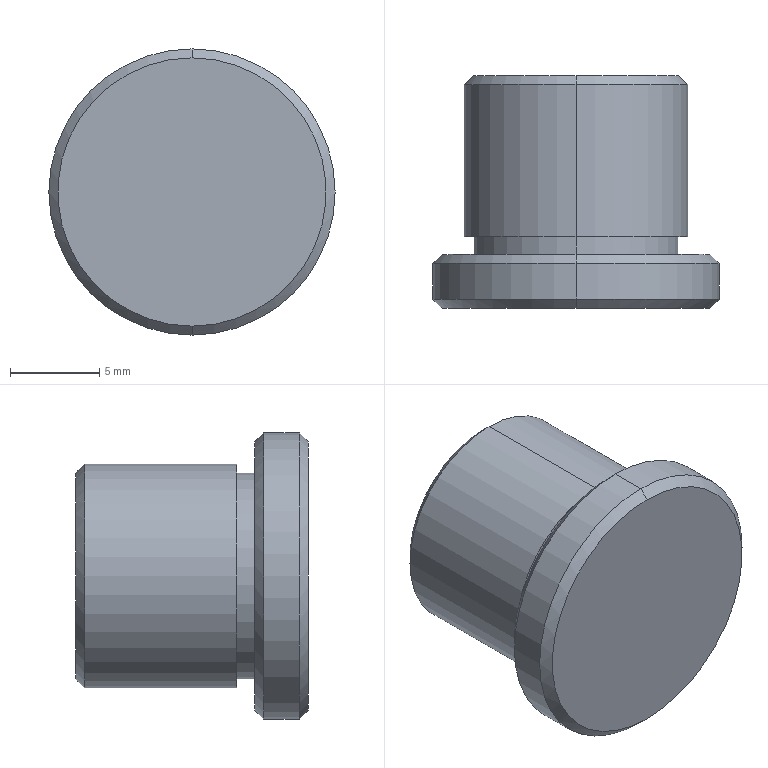Part | SolidWorks | features Chamfer 1, Revolution 1 | 1 solid | 16 faces | box 16 x 13 x 16 mm | volume 1794 mm3 | cone 6 | cylinder 6 | plane 4 | commonest cylinder face diameters 11.5 x2 12.5 x2 16 x2
STEP:
#1=CARTESIAN_POINT('',(74.024,-118.5,5.75));
#2=VERTEX_POINT('',#1);
#3=CARTESIAN_POINT('',(74.024,-118.5,-5.75));
#4=VERTEX_POINT('',#3);
#5=CARTESIAN_POINT('',(74.024,-118.5,0.));
#6=DIRECTION('',(0.,1.,0.));
#7=DIRECTION('',(0.,0.,-1.));
#8=AXIS2_PLACEMENT_3D('',#5,#6,#7);
#9=CIRCLE('',#8,5.75);
#10=EDGE_CURVE('',#2,#4,#9,.T.);
#11=ORIENTED_EDGE('',*,*,#10,.F.);
#12=CARTESIAN_POINT('',(74.024,-119.,6.25));
#13=VERTEX_POINT('',#12);
#14=CARTESIAN_POINT('',(74.024,-118.5,5.75));
#15=DIRECTION('',(0.,-0.7071,0.7071));
#16=VECTOR('',#15,1000.);
#17=LINE('',#14,#16);
#18=EDGE_CURVE('',#2,#13,#17,.T.);
#19=ORIENTED_EDGE('',*,*,#18,.T.);
#20=CARTESIAN_POINT('',(74.024,-119.,-6.25));
#21=VERTEX_POINT('',#20);
#22=CARTESIAN_POINT('',(74.024,-119.,0.));
#23=DIRECTION('',(0.,-1.,0.));
#24=DIRECTION('',(0.,0.,-1.));
#25=AXIS2_PLACEMENT_3D('',#22,#23,#24);
#26=CIRCLE('',#25,6.25);
#27=EDGE_CURVE('',#21,#13,#26,.T.);
#28=ORIENTED_EDGE('',*,*,#27,.F.);
#29=CARTESIAN_POINT('',(74.024,-118.5,-5.75));
#30=DIRECTION('',(0.,-0.7071,-0.7071));
#31=VECTOR('',#30,1000.);
#32=LINE('',#29,#31);
#33=EDGE_CURVE('',#4,#21,#32,.T.);
#34=ORIENTED_EDGE('',*,*,#33,.F.);
#35=EDGE_LOOP('',(#11,#19,#28,#34));
#36=FACE_OUTER_BOUND('',#35,.T.);
#37=CARTESIAN_POINT('',(74.024,-118.5,0.));
#38=DIRECTION('',(0.,-1.,0.));
#39=DIRECTION('',(0.,0.,-1.));
#40=AXIS2_PLACEMENT_3D('',#37,#38,#39);
#41=CONICAL_SURFACE('',#40,5.75,0.7854);
#42=ADVANCED_FACE('',(#36),#41,.T.);
#43=CARTESIAN_POINT('',(74.024,-131.5,-7.5));
#44=VERTEX_POINT('',#43);
#45=CARTESIAN_POINT('',(74.024,-131.5,7.5));
#46=VERTEX_POINT('',#45);
#47=CARTESIAN_POINT('',(74.024,-131.5,0.));
#48=DIRECTION('',(0.,-1.,0.));
#49=DIRECTION('',(0.,0.,1.));
#50=AXIS2_PLACEMENT_3D('',#47,#48,#49);
#51=CIRCLE('',#50,7.5);
#52=EDGE_CURVE('',#44,#46,#51,.T.);
#53=ORIENTED_EDGE('',*,*,#52,.F.);
#54=CARTESIAN_POINT('',(74.024,-131.,-8.));
#55=VERTEX_POINT('',#54);
#56=CARTESIAN_POINT('',(74.024,-131.,-8.));
#57=DIRECTION('',(0.,0.7071,-0.7071));
#58=VECTOR('',#57,1000.);
#59=LINE('',#56,#58);
#60=EDGE_CURVE('',#44,#55,#59,.T.);
#61=ORIENTED_EDGE('',*,*,#60,.T.);
#62=CARTESIAN_POINT('',(74.024,-131.,8.));
#63=VERTEX_POINT('',#62);
#64=CARTESIAN_POINT('',(74.024,-131.,0.));
#65=DIRECTION('',(0.,1.,0.));
#66=DIRECTION('',(0.,0.,1.));
#67=AXIS2_PLACEMENT_3D('',#64,#65,#66);
#68=CIRCLE('',#67,8.);
#69=EDGE_CURVE('',#63,#55,#68,.T.);
#70=ORIENTED_EDGE('',*,*,#69,.F.);
#71=CARTESIAN_POINT('',(74.024,-131.,8.));
#72=DIRECTION('',(0.,0.7071,0.7071));
#73=VECTOR('',#72,1000.);
#74=LINE('',#71,#73);
#75=EDGE_CURVE('',#46,#63,#74,.T.);
#76=ORIENTED_EDGE('',*,*,#75,.F.);
#77=EDGE_LOOP('',(#53,#61,#70,#76));
#78=FACE_OUTER_BOUND('',#77,.T.);
#79=CARTESIAN_POINT('',(74.024,-131.,0.));
#80=DIRECTION('',(0.,1.,0.));
#81=DIRECTION('',(0.,0.,1.));
#82=AXIS2_PLACEMENT_3D('',#79,#80,#81);
#83=CONICAL_SURFACE('',#82,8.,0.7854);
#84=ADVANCED_FACE('',(#78),#83,.T.);
#85=CARTESIAN_POINT('',(74.024,-128.5,7.5));
#86=VERTEX_POINT('',#85);
#87=CARTESIAN_POINT('',(74.024,-128.5,-7.5));
#88=VERTEX_POINT('',#87);
#89=CARTESIAN_POINT('',(74.024,-128.5,0.));
#90=DIRECTION('',(0.,1.,0.));
#91=DIRECTION('',(0.,0.,-1.));
#92=AXIS2_PLACEMENT_3D('',#89,#90,#91);
#93=CIRCLE('',#92,7.5);
#94=EDGE_CURVE('',#86,#88,#93,.T.);
#95=ORIENTED_EDGE('',*,*,#94,.F.);
#96=CARTESIAN_POINT('',(74.024,-129.,8.));
#97=VERTEX_POINT('',#96);
#98=CARTESIAN_POINT('',(74.024,-128.5,7.5));
#99=DIRECTION('',(0.,-0.7071,0.7071));
#100=VECTOR('',#99,1000.);
#101=LINE('',#98,#100);
#102=EDGE_CURVE('',#86,#97,#101,.T.);
#103=ORIENTED_EDGE('',*,*,#102,.T.);
#104=CARTESIAN_POINT('',(74.024,-129.,-8.));
#105=VERTEX_POINT('',#104);
#106=CARTESIAN_POINT('',(74.024,-129.,0.));
#107=DIRECTION('',(0.,-1.,0.));
#108=DIRECTION('',(0.,0.,-1.));
#109=AXIS2_PLACEMENT_3D('',#106,#107,#108);
#110=CIRCLE('',#109,8.);
#111=EDGE_CURVE('',#105,#97,#110,.T.);
#112=ORIENTED_EDGE('',*,*,#111,.F.);
#113=CARTESIAN_POINT('',(74.024,-128.5,-7.5));
#114=DIRECTION('',(0.,-0.7071,-0.7071));
#115=VECTOR('',#114,1000.);
#116=LINE('',#113,#115);
#117=EDGE_CURVE('',#88,#105,#116,.T.);
#118=ORIENTED_EDGE('',*,*,#117,.F.);
#119=EDGE_LOOP('',(#95,#103,#112,#118));
#120=FACE_OUTER_BOUND('',#119,.T.);
#121=CARTESIAN_POINT('',(74.024,-128.5,0.));
#122=DIRECTION('',(0.,-1.,0.));
#123=DIRECTION('',(0.,0.,-1.));
#124=AXIS2_PLACEMENT_3D('',#121,#122,#123);
#125=CONICAL_SURFACE('',#124,7.5,0.7854);
#126=ADVANCED_FACE('',(#120),#125,.T.);
#127=CARTESIAN_POINT('',(74.024,-128.5,5.75));
#128=VERTEX_POINT('',#127);
#129=CARTESIAN_POINT('',(74.024,-128.5,-5.75));
#130=VERTEX_POINT('',#129);
#131=CARTESIAN_POINT('',(74.024,-128.5,0.));
#132=DIRECTION('',(0.,1.,0.));
#133=DIRECTION('',(0.,0.,1.));
#134=AXIS2_PLACEMENT_3D('',#131,#132,#133);
#135=CIRCLE('',#134,5.75);
#136=EDGE_CURVE('',#128,#130,#135,.T.);
#137=ORIENTED_EDGE('',*,*,#136,.T.);
#138=CARTESIAN_POINT('',(74.024,-127.5,-5.75));
#139=VERTEX_POINT('',#138);
#140=CARTESIAN_POINT('',(74.024,-118.5,-5.75));
#141=DIRECTION('',(0.,1.,0.));
#142=VECTOR('',#141,1000.);
#143=LINE('',#140,#142);
#144=EDGE_CURVE('',#130,#139,#143,.T.);
#145=ORIENTED_EDGE('',*,*,#144,.T.);
#146=CARTESIAN_POINT('',(74.024,-127.5,5.75));
#147=VERTEX_POINT('',#146);
#148=CARTESIAN_POINT('',(74.024,-127.5,0.));
#149=DIRECTION('',(0.,1.,0.));
#150=DIRECTION('',(0.,0.,1.));
#151=AXIS2_PLACEMENT_3D('',#148,#149,#150);
#152=CIRCLE('',#151,5.75);
#153=EDGE_CURVE('',#147,#139,#152,.T.);
#154=ORIENTED_EDGE('',*,*,#153,.F.);
#155=CARTESIAN_POINT('',(74.024,-118.5,5.75));
#156=DIRECTION('',(0.,1.,0.));
#157=VECTOR('',#156,1000.);
#158=LINE('',#155,#157);
#159=EDGE_CURVE('',#128,#147,#158,.T.);
#160=ORIENTED_EDGE('',*,*,#159,.F.);
#161=EDGE_LOOP('',(#137,#145,#154,#160));
#162=FACE_OUTER_BOUND('',#161,.T.);
#163=CARTESIAN_POINT('',(74.024,-118.5,0.));
#164=DIRECTION('',(0.,1.,0.));
#165=DIRECTION('',(0.,0.,1.));
#166=AXIS2_PLACEMENT_3D('',#163,#164,#165);
#167=CYLINDRICAL_SURFACE('',#166,5.75);
#168=ADVANCED_FACE('',(#162),#167,.T.);
#169=CARTESIAN_POINT('',(74.024,-127.5,6.25));
#170=VERTEX_POINT('',#169);
#171=CARTESIAN_POINT('',(74.024,-127.5,-6.25));
#172=VERTEX_POINT('',#171);
#173=CARTESIAN_POINT('',(74.024,-127.5,0.));
#174=DIRECTION('',(0.,1.,0.));
#175=DIRECTION('',(0.,0.,1.));
#176=AXIS2_PLACEMENT_3D('',#173,#174,#175);
#177=CIRCLE('',#176,6.25);
#178=EDGE_CURVE('',#170,#172,#177,.T.);
#179=ORIENTED_EDGE('',*,*,#178,.T.);
#180=CARTESIAN_POINT('',(74.024,-118.5,-6.25));
#181=DIRECTION('',(0.,1.,0.));
#182=VECTOR('',#181,1000.);
#183=LINE('',#180,#182);
#184=EDGE_CURVE('',#172,#21,#183,.T.);
#185=ORIENTED_EDGE('',*,*,#184,.T.);
#186=ORIENTED_EDGE('',*,*,#27,.T.);
#187=CARTESIAN_POINT('',(74.024,-118.5,6.25));
#188=DIRECTION('',(0.,1.,0.));
#189=VECTOR('',#188,1000.);
#190=LINE('',#187,#189);
#191=EDGE_CURVE('',#170,#13,#190,.T.);
#192=ORIENTED_EDGE('',*,*,#191,.F.);
#193=EDGE_LOOP('',(#179,#185,#186,#192));
#194=FACE_OUTER_BOUND('',#193,.T.);
#195=CARTESIAN_POINT('',(74.024,-118.5,0.));
#196=DIRECTION('',(0.,1.,0.));
#197=DIRECTION('',(0.,0.,1.));
#198=AXIS2_PLACEMENT_3D('',#195,#196,#197);
#199=CYLINDRICAL_SURFACE('',#198,6.25);
#200=ADVANCED_FACE('',(#194),#199,.T.);
#201=ORIENTED_EDGE('',*,*,#69,.T.);
#202=CARTESIAN_POINT('',(74.024,-118.5,-8.));
#203=DIRECTION('',(0.,1.,0.));
#204=VECTOR('',#203,1000.);
#205=LINE('',#202,#204);
#206=EDGE_CURVE('',#55,#105,#205,.T.);
#207=ORIENTED_EDGE('',*,*,#206,.T.);
#208=ORIENTED_EDGE('',*,*,#111,.T.);
#209=CARTESIAN_POINT('',(74.024,-118.5,8.));
#210=DIRECTION('',(0.,1.,0.));
#211=VECTOR('',#210,1000.);
#212=LINE('',#209,#211);
#213=EDGE_CURVE('',#63,#97,#212,.T.);
#214=ORIENTED_EDGE('',*,*,#213,.F.);
#215=EDGE_LOOP('',(#201,#207,#208,#214));
#216=FACE_OUTER_BOUND('',#215,.T.);
#217=CARTESIAN_POINT('',(74.024,-118.5,0.));
#218=DIRECTION('',(0.,1.,0.));
#219=DIRECTION('',(0.,0.,1.));
#220=AXIS2_PLACEMENT_3D('',#217,#218,#219);
#221=CYLINDRICAL_SURFACE('',#220,8.);
#222=ADVANCED_FACE('',(#216),#221,.T.);
#223=ORIENTED_EDGE('',*,*,#206,.F.);
#224=CARTESIAN_POINT('',(74.024,-131.,0.));
#225=DIRECTION('',(0.,1.,0.));
#226=DIRECTION('',(0.,0.,1.));
#227=AXIS2_PLACEMENT_3D('',#224,#225,#226);
#228=CIRCLE('',#227,8.);
#229=EDGE_CURVE('',#55,#63,#228,.T.);
#230=ORIENTED_EDGE('',*,*,#229,.T.);
#231=ORIENTED_EDGE('',*,*,#213,.T.);
#232=CARTESIAN_POINT('',(74.024,-129.,0.));
#233=DIRECTION('',(0.,-1.,0.));
#234=DIRECTION('',(0.,0.,-1.));
#235=AXIS2_PLACEMENT_3D('',#232,#233,#234);
#236=CIRCLE('',#235,8.);
#237=EDGE_CURVE('',#97,#105,#236,.T.);
#238=ORIENTED_EDGE('',*,*,#237,.T.);
#239=EDGE_LOOP('',(#223,#230,#231,#238));
#240=FACE_OUTER_BOUND('',#239,.T.);
#241=CARTESIAN_POINT('',(74.024,-118.5,0.));
#242=DIRECTION('',(0.,1.,0.));
#243=DIRECTION('',(0.,0.,1.));
#244=AXIS2_PLACEMENT_3D('',#241,#242,#243);
#245=CYLINDRICAL_SURFACE('',#244,8.);
#246=ADVANCED_FACE('',(#240),#245,.T.);
#247=CARTESIAN_POINT('',(74.024,-131.5,0.));
#248=DIRECTION('',(0.,-1.,0.));
#249=DIRECTION('',(0.,0.,1.));
#250=AXIS2_PLACEMENT_3D('',#247,#248,#249);
#251=CIRCLE('',#250,7.5);
#252=EDGE_CURVE('',#46,#44,#251,.T.);
#253=ORIENTED_EDGE('',*,*,#252,.T.);
#254=ORIENTED_EDGE('',*,*,#52,.T.);
#255=EDGE_LOOP('',(#253,#254));
#256=FACE_OUTER_BOUND('',#255,.T.);
#257=CARTESIAN_POINT('',(82.024,-131.5,0.));
#258=DIRECTION('',(0.,1.,0.));
#259=DIRECTION('',(0.,0.,1.));
#260=AXIS2_PLACEMENT_3D('',#257,#258,#259);
#261=PLANE('',#260);
#262=ADVANCED_FACE('',(#256),#261,.F.);
#263=CARTESIAN_POINT('',(74.024,-118.5,0.));
#264=DIRECTION('',(0.,1.,0.));
#265=DIRECTION('',(0.,0.,-1.));
#266=AXIS2_PLACEMENT_3D('',#263,#264,#265);
#267=CIRCLE('',#266,5.75);
#268=EDGE_CURVE('',#4,#2,#267,.T.);
#269=ORIENTED_EDGE('',*,*,#268,.T.);
#270=ORIENTED_EDGE('',*,*,#10,.T.);
#271=EDGE_LOOP('',(#269,#270));
#272=FACE_OUTER_BOUND('',#271,.T.);
#273=CARTESIAN_POINT('',(80.274,-118.5,0.));
#274=DIRECTION('',(0.,-1.,0.));
#275=DIRECTION('',(0.,0.,-1.));
#276=AXIS2_PLACEMENT_3D('',#273,#274,#275);
#277=PLANE('',#276);
#278=ADVANCED_FACE('',(#272),#277,.F.);
#279=ORIENTED_EDGE('',*,*,#184,.F.);
#280=CARTESIAN_POINT('',(74.024,-127.5,0.));
#281=DIRECTION('',(0.,1.,0.));
#282=DIRECTION('',(0.,0.,1.));
#283=AXIS2_PLACEMENT_3D('',#280,#281,#282);
#284=CIRCLE('',#283,6.25);
#285=EDGE_CURVE('',#172,#170,#284,.T.);
#286=ORIENTED_EDGE('',*,*,#285,.T.);
#287=ORIENTED_EDGE('',*,*,#191,.T.);
#288=CARTESIAN_POINT('',(74.024,-119.,0.));
#289=DIRECTION('',(0.,-1.,0.));
#290=DIRECTION('',(0.,0.,-1.));
#291=AXIS2_PLACEMENT_3D('',#288,#289,#290);
#292=CIRCLE('',#291,6.25);
#293=EDGE_CURVE('',#13,#21,#292,.T.);
#294=ORIENTED_EDGE('',*,*,#293,.T.);
#295=EDGE_LOOP('',(#279,#286,#287,#294));
#296=FACE_OUTER_BOUND('',#295,.T.);
#297=CARTESIAN_POINT('',(74.024,-118.5,0.));
#298=DIRECTION('',(0.,1.,0.));
#299=DIRECTION('',(0.,0.,1.));
#300=AXIS2_PLACEMENT_3D('',#297,#298,#299);
#301=CYLINDRICAL_SURFACE('',#300,6.25);
#302=ADVANCED_FACE('',(#296),#301,.T.);
#303=ORIENTED_EDGE('',*,*,#178,.F.);
#304=ORIENTED_EDGE('',*,*,#285,.F.);
#305=EDGE_LOOP('',(#303,#304));
#306=FACE_OUTER_BOUND('',#305,.T.);
#307=ORIENTED_EDGE('',*,*,#153,.T.);
#308=CARTESIAN_POINT('',(74.024,-127.5,0.));
#309=DIRECTION('',(0.,1.,0.));
#310=DIRECTION('',(0.,0.,1.));
#311=AXIS2_PLACEMENT_3D('',#308,#309,#310);
#312=CIRCLE('',#311,5.75);
#313=EDGE_CURVE('',#139,#147,#312,.T.);
#314=ORIENTED_EDGE('',*,*,#313,.T.);
#315=EDGE_LOOP('',(#307,#314));
#316=FACE_BOUND('',#315,.T.);
#317=CARTESIAN_POINT('',(80.274,-127.5,0.));
#318=DIRECTION('',(0.,1.,0.));
#319=DIRECTION('',(0.,0.,1.));
#320=AXIS2_PLACEMENT_3D('',#317,#318,#319);
#321=PLANE('',#320);
#322=ADVANCED_FACE('',(#306,#316),#321,.F.);
#323=ORIENTED_EDGE('',*,*,#144,.F.);
#324=CARTESIAN_POINT('',(74.024,-128.5,0.));
#325=DIRECTION('',(0.,1.,0.));
#326=DIRECTION('',(0.,0.,1.));
#327=AXIS2_PLACEMENT_3D('',#324,#325,#326);
#328=CIRCLE('',#327,5.75);
#329=EDGE_CURVE('',#130,#128,#328,.T.);
#330=ORIENTED_EDGE('',*,*,#329,.T.);
#331=ORIENTED_EDGE('',*,*,#159,.T.);
#332=ORIENTED_EDGE('',*,*,#313,.F.);
#333=EDGE_LOOP('',(#323,#330,#331,#332));
#334=FACE_OUTER_BOUND('',#333,.T.);
#335=CARTESIAN_POINT('',(74.024,-118.5,0.));
#336=DIRECTION('',(0.,1.,0.));
#337=DIRECTION('',(0.,0.,1.));
#338=AXIS2_PLACEMENT_3D('',#335,#336,#337);
#339=CYLINDRICAL_SURFACE('',#338,5.75);
#340=ADVANCED_FACE('',(#334),#339,.T.);
#341=CARTESIAN_POINT('',(74.024,-128.5,0.));
#342=DIRECTION('',(0.,1.,0.));
#343=DIRECTION('',(0.,0.,-1.));
#344=AXIS2_PLACEMENT_3D('',#341,#342,#343);
#345=CIRCLE('',#344,7.5);
#346=EDGE_CURVE('',#88,#86,#345,.T.);
#347=ORIENTED_EDGE('',*,*,#346,.T.);
#348=ORIENTED_EDGE('',*,*,#94,.T.);
#349=EDGE_LOOP('',(#347,#348));
#350=FACE_OUTER_BOUND('',#349,.T.);
#351=ORIENTED_EDGE('',*,*,#136,.F.);
#352=ORIENTED_EDGE('',*,*,#329,.F.);
#353=EDGE_LOOP('',(#351,#352));
#354=FACE_BOUND('',#353,.T.);
#355=CARTESIAN_POINT('',(82.024,-128.5,0.));
#356=DIRECTION('',(0.,-1.,0.));
#357=DIRECTION('',(0.,0.,-1.));
#358=AXIS2_PLACEMENT_3D('',#355,#356,#357);
#359=PLANE('',#358);
#360=ADVANCED_FACE('',(#350,#354),#359,.F.);
#361=ORIENTED_EDGE('',*,*,#102,.F.);
#362=ORIENTED_EDGE('',*,*,#346,.F.);
#363=ORIENTED_EDGE('',*,*,#117,.T.);
#364=ORIENTED_EDGE('',*,*,#237,.F.);
#365=EDGE_LOOP('',(#361,#362,#363,#364));
#366=FACE_OUTER_BOUND('',#365,.T.);
#367=CARTESIAN_POINT('',(74.024,-128.5,0.));
#368=DIRECTION('',(0.,-1.,0.));
#369=DIRECTION('',(0.,0.,-1.));
#370=AXIS2_PLACEMENT_3D('',#367,#368,#369);
#371=CONICAL_SURFACE('',#370,7.5,0.7854);
#372=ADVANCED_FACE('',(#366),#371,.T.);
#373=ORIENTED_EDGE('',*,*,#60,.F.);
#374=ORIENTED_EDGE('',*,*,#252,.F.);
#375=ORIENTED_EDGE('',*,*,#75,.T.);
#376=ORIENTED_EDGE('',*,*,#229,.F.);
#377=EDGE_LOOP('',(#373,#374,#375,#376));
#378=FACE_OUTER_BOUND('',#377,.T.);
#379=CARTESIAN_POINT('',(74.024,-131.,0.));
#380=DIRECTION('',(0.,1.,0.));
#381=DIRECTION('',(0.,0.,1.));
#382=AXIS2_PLACEMENT_3D('',#379,#380,#381);
#383=CONICAL_SURFACE('',#382,8.,0.7854);
#384=ADVANCED_FACE('',(#378),#383,.T.);
#385=ORIENTED_EDGE('',*,*,#18,.F.);
#386=ORIENTED_EDGE('',*,*,#268,.F.);
#387=ORIENTED_EDGE('',*,*,#33,.T.);
#388=ORIENTED_EDGE('',*,*,#293,.F.);
#389=EDGE_LOOP('',(#385,#386,#387,#388));
#390=FACE_OUTER_BOUND('',#389,.T.);
#391=CARTESIAN_POINT('',(74.024,-118.5,0.));
#392=DIRECTION('',(0.,-1.,0.));
#393=DIRECTION('',(0.,0.,-1.));
#394=AXIS2_PLACEMENT_3D('',#391,#392,#393);
#395=CONICAL_SURFACE('',#394,5.75,0.7854);
#396=ADVANCED_FACE('',(#390),#395,.T.);
#397=CLOSED_SHELL('',(#42,#84,#126,#168,#200,#222,#246,#262,#278,#302,#322,#340,#360,#372,#384,#396));
#398=MANIFOLD_SOLID_BREP('',#397);
#399=CARTESIAN_POINT('',(0.,0.,0.));
#400=DIRECTION('',(0.,0.,1.));
#401=DIRECTION('',(1.,0.,0.));
#402=AXIS2_PLACEMENT_3D('',#399,#400,#401);
#403=(LENGTH_UNIT()NAMED_UNIT(*)SI_UNIT(.MILLI.,.METRE.));
#404=UNCERTAINTY_MEASURE_WITH_UNIT(LENGTH_MEASURE(0.00001),#403,'','');
#405=(NAMED_UNIT(*)PLANE_ANGLE_UNIT()SI_UNIT($,.RADIAN.));
#406=(NAMED_UNIT(*)SI_UNIT($,.STERADIAN.)SOLID_ANGLE_UNIT());
#407=(GEOMETRIC_REPRESENTATION_CONTEXT(3)GLOBAL_UNCERTAINTY_ASSIGNED_CONTEXT((#404))GLOBAL_UNIT_ASSIGNED_CONTEXT((#403,#405,#406))REPRESENTATION_CONTEXT('',''));
#408=ADVANCED_BREP_SHAPE_REPRESENTATION('',(#398,#402),#407);